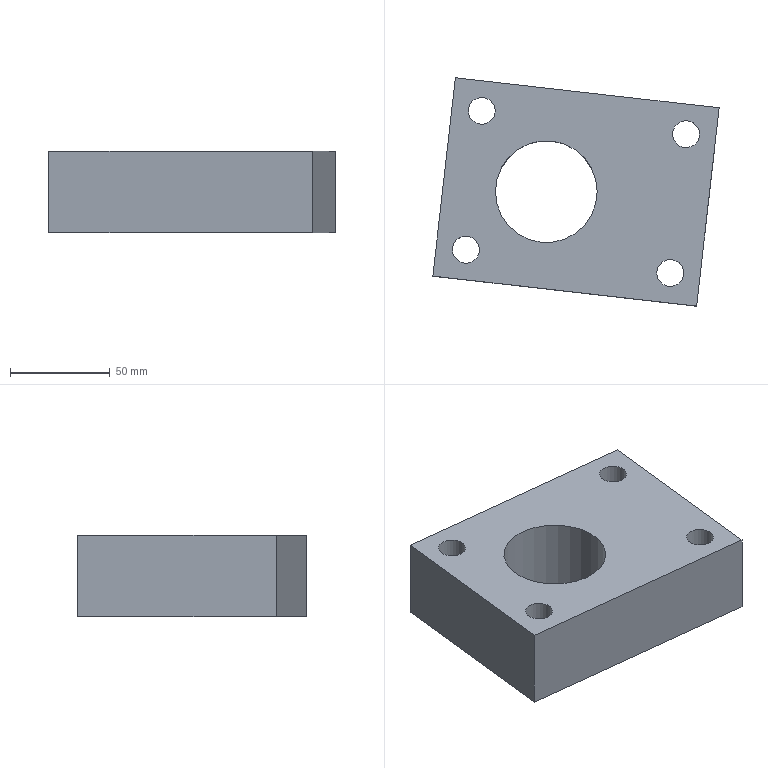Part | NX | features solid 2 | 1 solid | 19 faces | box 143.465 x 114.413 x 41 mm | volume 427808 mm3 | plane 10 | cylinder 9 | commonest cylinder face diameters 13.5 x4 20 x4 51 x1
STEP:
#1=CARTESIAN_POINT('',(2599.823,-120.761,101.));
#2=VERTEX_POINT('',#1);
#3=CARTESIAN_POINT('',(2593.073,-120.761,101.));
#4=DIRECTION('',(0.,0.,-1.));
#5=DIRECTION('',(1.,0.,0.));
#6=AXIS2_PLACEMENT_3D('',#3,#4,#5);
#7=CIRCLE('',#6,6.75);
#8=EDGE_CURVE('',#2,#2,#7,.T.);
#9=ORIENTED_EDGE('',*,*,#8,.T.);
#10=EDGE_LOOP('',(#9));
#11=FACE_BOUND('',#10,.T.);
#12=CARTESIAN_POINT('',(2607.575,-52.73,101.));
#13=VERTEX_POINT('',#12);
#14=CARTESIAN_POINT('',(2600.998,-51.211,101.));
#15=DIRECTION('',(0.,0.,1.));
#16=DIRECTION('',(0.9744,-0.225,0.));
#17=AXIS2_PLACEMENT_3D('',#14,#15,#16);
#18=CIRCLE('',#17,6.75);
#19=EDGE_CURVE('',#13,#13,#18,.T.);
#20=ORIENTED_EDGE('',*,*,#19,.F.);
#21=EDGE_LOOP('',(#20));
#22=FACE_BOUND('',#21,.T.);
#23=CARTESIAN_POINT('',(2606.279,-137.363,101.));
#24=VERTEX_POINT('',#23);
#25=CARTESIAN_POINT('',(2474.134,-122.307,101.));
#26=VERTEX_POINT('',#25);
#27=CARTESIAN_POINT('',(2529.774,-128.646,101.));
#28=DIRECTION('',(-0.9936,0.1132,0.));
#29=VECTOR('',#28,1000.);
#30=LINE('',#27,#29);
#31=EDGE_CURVE('',#24,#26,#30,.T.);
#32=ORIENTED_EDGE('',*,*,#31,.F.);
#33=CARTESIAN_POINT('',(2617.599,-38.006,101.));
#34=VERTEX_POINT('',#33);
#35=CARTESIAN_POINT('',(2612.505,-82.717,101.));
#36=DIRECTION('',(-0.1132,-0.9936,0.));
#37=VECTOR('',#36,1000.);
#38=LINE('',#35,#37);
#39=EDGE_CURVE('',#34,#24,#38,.T.);
#40=ORIENTED_EDGE('',*,*,#39,.F.);
#41=CARTESIAN_POINT('',(2485.454,-22.95,101.));
#42=VERTEX_POINT('',#41);
#43=CARTESIAN_POINT('',(2541.094,-29.289,101.));
#44=DIRECTION('',(0.9936,-0.1132,0.));
#45=VECTOR('',#44,1000.);
#46=LINE('',#43,#45);
#47=EDGE_CURVE('',#42,#34,#46,.T.);
#48=ORIENTED_EDGE('',*,*,#47,.F.);
#49=CARTESIAN_POINT('',(2480.36,-67.661,101.));
#50=DIRECTION('',(0.1132,0.9936,0.));
#51=VECTOR('',#50,1000.);
#52=LINE('',#49,#51);
#53=EDGE_CURVE('',#26,#42,#52,.T.);
#54=ORIENTED_EDGE('',*,*,#53,.F.);
#55=EDGE_LOOP('',(#32,#40,#48,#54));
#56=FACE_BOUND('',#55,.T.);
#57=CARTESIAN_POINT('',(2556.5,-80.,101.));
#58=VERTEX_POINT('',#57);
#59=CARTESIAN_POINT('',(2531.,-80.,101.));
#60=DIRECTION('',(0.,0.,1.));
#61=DIRECTION('',(1.,0.,0.));
#62=AXIS2_PLACEMENT_3D('',#59,#60,#61);
#63=CIRCLE('',#62,25.5);
#64=EDGE_CURVE('',#58,#58,#63,.T.);
#65=ORIENTED_EDGE('',*,*,#64,.F.);
#66=EDGE_LOOP('',(#65));
#67=FACE_BOUND('',#66,.T.);
#68=CARTESIAN_POINT('',(2484.158,-107.583,101.));
#69=VERTEX_POINT('',#68);
#70=CARTESIAN_POINT('',(2490.735,-109.102,101.));
#71=DIRECTION('',(0.,0.,1.));
#72=DIRECTION('',(-0.9744,0.225,0.));
#73=AXIS2_PLACEMENT_3D('',#70,#71,#72);
#74=CIRCLE('',#73,6.75);
#75=EDGE_CURVE('',#69,#69,#74,.T.);
#76=ORIENTED_EDGE('',*,*,#75,.F.);
#77=EDGE_LOOP('',(#76));
#78=FACE_BOUND('',#77,.T.);
#79=CARTESIAN_POINT('',(2491.91,-39.552,101.));
#80=VERTEX_POINT('',#79);
#81=CARTESIAN_POINT('',(2498.66,-39.552,101.));
#82=DIRECTION('',(0.,0.,-1.));
#83=DIRECTION('',(-1.,0.,0.));
#84=AXIS2_PLACEMENT_3D('',#81,#82,#83);
#85=CIRCLE('',#84,6.75);
#86=EDGE_CURVE('',#80,#80,#85,.T.);
#87=ORIENTED_EDGE('',*,*,#86,.T.);
#88=EDGE_LOOP('',(#87));
#89=FACE_BOUND('',#88,.T.);
#90=CARTESIAN_POINT('',(282.5,193.,101.));
#91=DIRECTION('',(0.,0.,1.));
#92=DIRECTION('',(-1.,0.,0.));
#93=AXIS2_PLACEMENT_3D('',#90,#91,#92);
#94=PLANE('',#93);
#95=ADVANCED_FACE('',(#11,#22,#56,#67,#78,#89),#94,.T.);
#96=CARTESIAN_POINT('',(2603.073,-120.761,60.));
#97=VERTEX_POINT('',#96);
#98=CARTESIAN_POINT('',(2593.073,-120.761,60.));
#99=DIRECTION('',(0.,0.,1.));
#100=DIRECTION('',(1.,0.,0.));
#101=AXIS2_PLACEMENT_3D('',#98,#99,#100);
#102=CIRCLE('',#101,10.);
#103=EDGE_CURVE('',#97,#97,#102,.T.);
#104=ORIENTED_EDGE('',*,*,#103,.T.);
#105=EDGE_LOOP('',(#104));
#106=FACE_BOUND('',#105,.T.);
#107=CARTESIAN_POINT('',(2610.741,-53.461,60.));
#108=VERTEX_POINT('',#107);
#109=CARTESIAN_POINT('',(2600.998,-51.211,60.));
#110=DIRECTION('',(0.,0.,-1.));
#111=DIRECTION('',(0.9744,-0.225,0.));
#112=AXIS2_PLACEMENT_3D('',#109,#110,#111);
#113=CIRCLE('',#112,10.);
#114=EDGE_CURVE('',#108,#108,#113,.T.);
#115=ORIENTED_EDGE('',*,*,#114,.F.);
#116=EDGE_LOOP('',(#115));
#117=FACE_BOUND('',#116,.T.);
#118=CARTESIAN_POINT('',(2606.279,-137.363,60.));
#119=VERTEX_POINT('',#118);
#120=CARTESIAN_POINT('',(2617.599,-38.006,60.));
#121=VERTEX_POINT('',#120);
#122=CARTESIAN_POINT('',(2612.505,-82.717,60.));
#123=DIRECTION('',(0.1132,0.9936,0.));
#124=VECTOR('',#123,1000.);
#125=LINE('',#122,#124);
#126=EDGE_CURVE('',#119,#121,#125,.T.);
#127=ORIENTED_EDGE('',*,*,#126,.F.);
#128=CARTESIAN_POINT('',(2474.134,-122.307,60.));
#129=VERTEX_POINT('',#128);
#130=CARTESIAN_POINT('',(2529.774,-128.646,60.));
#131=DIRECTION('',(0.9936,-0.1132,0.));
#132=VECTOR('',#131,1000.);
#133=LINE('',#130,#132);
#134=EDGE_CURVE('',#129,#119,#133,.T.);
#135=ORIENTED_EDGE('',*,*,#134,.F.);
#136=CARTESIAN_POINT('',(2485.454,-22.95,60.));
#137=VERTEX_POINT('',#136);
#138=CARTESIAN_POINT('',(2480.36,-67.661,60.));
#139=DIRECTION('',(-0.1132,-0.9936,0.));
#140=VECTOR('',#139,1000.);
#141=LINE('',#138,#140);
#142=EDGE_CURVE('',#137,#129,#141,.T.);
#143=ORIENTED_EDGE('',*,*,#142,.F.);
#144=CARTESIAN_POINT('',(2541.094,-29.289,60.));
#145=DIRECTION('',(-0.9936,0.1132,0.));
#146=VECTOR('',#145,1000.);
#147=LINE('',#144,#146);
#148=EDGE_CURVE('',#121,#137,#147,.T.);
#149=ORIENTED_EDGE('',*,*,#148,.F.);
#150=EDGE_LOOP('',(#127,#135,#143,#149));
#151=FACE_BOUND('',#150,.T.);
#152=CARTESIAN_POINT('',(2556.5,-80.,60.));
#153=VERTEX_POINT('',#152);
#154=CARTESIAN_POINT('',(2531.,-80.,60.));
#155=DIRECTION('',(0.,0.,-1.));
#156=DIRECTION('',(1.,0.,0.));
#157=AXIS2_PLACEMENT_3D('',#154,#155,#156);
#158=CIRCLE('',#157,25.5);
#159=EDGE_CURVE('',#153,#153,#158,.T.);
#160=ORIENTED_EDGE('',*,*,#159,.F.);
#161=EDGE_LOOP('',(#160));
#162=FACE_BOUND('',#161,.T.);
#163=CARTESIAN_POINT('',(2480.992,-106.852,60.));
#164=VERTEX_POINT('',#163);
#165=CARTESIAN_POINT('',(2490.735,-109.102,60.));
#166=DIRECTION('',(0.,0.,-1.));
#167=DIRECTION('',(-0.9744,0.225,0.));
#168=AXIS2_PLACEMENT_3D('',#165,#166,#167);
#169=CIRCLE('',#168,10.);
#170=EDGE_CURVE('',#164,#164,#169,.T.);
#171=ORIENTED_EDGE('',*,*,#170,.F.);
#172=EDGE_LOOP('',(#171));
#173=FACE_BOUND('',#172,.T.);
#174=CARTESIAN_POINT('',(2488.66,-39.552,60.));
#175=VERTEX_POINT('',#174);
#176=CARTESIAN_POINT('',(2498.66,-39.552,60.));
#177=DIRECTION('',(0.,0.,1.));
#178=DIRECTION('',(-1.,0.,0.));
#179=AXIS2_PLACEMENT_3D('',#176,#177,#178);
#180=CIRCLE('',#179,10.);
#181=EDGE_CURVE('',#175,#175,#180,.T.);
#182=ORIENTED_EDGE('',*,*,#181,.T.);
#183=EDGE_LOOP('',(#182));
#184=FACE_BOUND('',#183,.T.);
#185=CARTESIAN_POINT('',(2658.641,-285.511,60.));
#186=DIRECTION('',(0.,0.,1.));
#187=DIRECTION('',(-1.,0.,0.));
#188=AXIS2_PLACEMENT_3D('',#185,#186,#187);
#189=PLANE('',#188);
#190=ADVANCED_FACE('',(#106,#117,#151,#162,#173,#184),#189,.F.);
#191=CARTESIAN_POINT('',(2606.279,-137.363,-10.));
#192=DIRECTION('',(0.,0.,1.));
#193=VECTOR('',#192,1000.);
#194=LINE('',#191,#193);
#195=EDGE_CURVE('',#119,#24,#194,.T.);
#196=ORIENTED_EDGE('',*,*,#195,.T.);
#197=ORIENTED_EDGE('',*,*,#31,.T.);
#198=CARTESIAN_POINT('',(2474.134,-122.307,-10.));
#199=DIRECTION('',(0.,0.,1.));
#200=VECTOR('',#199,1000.);
#201=LINE('',#198,#200);
#202=EDGE_CURVE('',#129,#26,#201,.T.);
#203=ORIENTED_EDGE('',*,*,#202,.F.);
#204=ORIENTED_EDGE('',*,*,#134,.T.);
#205=EDGE_LOOP('',(#196,#197,#203,#204));
#206=FACE_BOUND('',#205,.T.);
#207=CARTESIAN_POINT('',(2529.774,-128.646,-10.));
#208=DIRECTION('',(-0.1132,-0.9936,0.));
#209=DIRECTION('',(-0.9936,0.1132,0.));
#210=AXIS2_PLACEMENT_3D('',#207,#208,#209);
#211=PLANE('',#210);
#212=ADVANCED_FACE('',(#206),#211,.T.);
#213=ORIENTED_EDGE('',*,*,#202,.T.);
#214=ORIENTED_EDGE('',*,*,#53,.T.);
#215=CARTESIAN_POINT('',(2485.454,-22.95,-10.));
#216=DIRECTION('',(0.,0.,1.));
#217=VECTOR('',#216,1000.);
#218=LINE('',#215,#217);
#219=EDGE_CURVE('',#137,#42,#218,.T.);
#220=ORIENTED_EDGE('',*,*,#219,.F.);
#221=ORIENTED_EDGE('',*,*,#142,.T.);
#222=EDGE_LOOP('',(#213,#214,#220,#221));
#223=FACE_BOUND('',#222,.T.);
#224=CARTESIAN_POINT('',(2480.36,-67.661,-10.));
#225=DIRECTION('',(-0.9936,0.1132,0.));
#226=DIRECTION('',(0.1132,0.9936,0.));
#227=AXIS2_PLACEMENT_3D('',#224,#225,#226);
#228=PLANE('',#227);
#229=ADVANCED_FACE('',(#223),#228,.T.);
#230=ORIENTED_EDGE('',*,*,#219,.T.);
#231=ORIENTED_EDGE('',*,*,#47,.T.);
#232=CARTESIAN_POINT('',(2617.599,-38.006,-10.));
#233=DIRECTION('',(0.,0.,1.));
#234=VECTOR('',#233,1000.);
#235=LINE('',#232,#234);
#236=EDGE_CURVE('',#121,#34,#235,.T.);
#237=ORIENTED_EDGE('',*,*,#236,.F.);
#238=ORIENTED_EDGE('',*,*,#148,.T.);
#239=EDGE_LOOP('',(#230,#231,#237,#238));
#240=FACE_BOUND('',#239,.T.);
#241=CARTESIAN_POINT('',(2541.094,-29.289,-10.));
#242=DIRECTION('',(0.1132,0.9936,0.));
#243=DIRECTION('',(0.9936,-0.1132,0.));
#244=AXIS2_PLACEMENT_3D('',#241,#242,#243);
#245=PLANE('',#244);
#246=ADVANCED_FACE('',(#240),#245,.T.);
#247=ORIENTED_EDGE('',*,*,#126,.T.);
#248=ORIENTED_EDGE('',*,*,#236,.T.);
#249=ORIENTED_EDGE('',*,*,#39,.T.);
#250=ORIENTED_EDGE('',*,*,#195,.F.);
#251=EDGE_LOOP('',(#247,#248,#249,#250));
#252=FACE_BOUND('',#251,.T.);
#253=CARTESIAN_POINT('',(2612.505,-82.717,-10.));
#254=DIRECTION('',(0.9936,-0.1132,0.));
#255=DIRECTION('',(-0.1132,-0.9936,0.));
#256=AXIS2_PLACEMENT_3D('',#253,#254,#255);
#257=PLANE('',#256);
#258=ADVANCED_FACE('',(#252),#257,.T.);
#259=ORIENTED_EDGE('',*,*,#64,.T.);
#260=EDGE_LOOP('',(#259));
#261=FACE_BOUND('',#260,.T.);
#262=ORIENTED_EDGE('',*,*,#159,.T.);
#263=EDGE_LOOP('',(#262));
#264=FACE_BOUND('',#263,.T.);
#265=CARTESIAN_POINT('',(2531.,-80.,-101.));
#266=DIRECTION('',(0.,0.,1.));
#267=DIRECTION('',(-1.,0.,0.));
#268=AXIS2_PLACEMENT_3D('',#265,#266,#267);
#269=CYLINDRICAL_SURFACE('',#268,25.5);
#270=ADVANCED_FACE('',(#261,#264),#269,.F.);
#271=CARTESIAN_POINT('',(2607.575,-52.73,75.));
#272=VERTEX_POINT('',#271);
#273=CARTESIAN_POINT('',(2600.998,-51.211,75.));
#274=DIRECTION('',(0.,0.,-1.));
#275=DIRECTION('',(0.9744,-0.225,0.));
#276=AXIS2_PLACEMENT_3D('',#273,#274,#275);
#277=CIRCLE('',#276,6.75);
#278=EDGE_CURVE('',#272,#272,#277,.T.);
#279=ORIENTED_EDGE('',*,*,#278,.T.);
#280=EDGE_LOOP('',(#279));
#281=FACE_BOUND('',#280,.T.);
#282=ORIENTED_EDGE('',*,*,#19,.T.);
#283=EDGE_LOOP('',(#282));
#284=FACE_BOUND('',#283,.T.);
#285=CARTESIAN_POINT('',(2600.998,-51.211,60.));
#286=DIRECTION('',(0.,0.,1.));
#287=DIRECTION('',(-0.9744,0.225,0.));
#288=AXIS2_PLACEMENT_3D('',#285,#286,#287);
#289=CYLINDRICAL_SURFACE('',#288,6.75);
#290=ADVANCED_FACE('',(#281,#284),#289,.F.);
#291=ORIENTED_EDGE('',*,*,#278,.F.);
#292=EDGE_LOOP('',(#291));
#293=FACE_BOUND('',#292,.T.);
#294=CARTESIAN_POINT('',(2610.741,-53.461,75.));
#295=VERTEX_POINT('',#294);
#296=CARTESIAN_POINT('',(2600.998,-51.211,75.));
#297=DIRECTION('',(0.,0.,-1.));
#298=DIRECTION('',(0.9744,-0.225,0.));
#299=AXIS2_PLACEMENT_3D('',#296,#297,#298);
#300=CIRCLE('',#299,10.);
#301=EDGE_CURVE('',#295,#295,#300,.T.);
#302=ORIENTED_EDGE('',*,*,#301,.T.);
#303=EDGE_LOOP('',(#302));
#304=FACE_BOUND('',#303,.T.);
#305=CARTESIAN_POINT('',(2600.998,-51.211,75.));
#306=DIRECTION('',(0.,0.,1.));
#307=DIRECTION('',(-0.9744,0.225,0.));
#308=AXIS2_PLACEMENT_3D('',#305,#306,#307);
#309=PLANE('',#308);
#310=ADVANCED_FACE('',(#293,#304),#309,.F.);
#311=ORIENTED_EDGE('',*,*,#301,.F.);
#312=EDGE_LOOP('',(#311));
#313=FACE_BOUND('',#312,.T.);
#314=ORIENTED_EDGE('',*,*,#114,.T.);
#315=EDGE_LOOP('',(#314));
#316=FACE_BOUND('',#315,.T.);
#317=CARTESIAN_POINT('',(2600.998,-51.211,60.));
#318=DIRECTION('',(0.,0.,1.));
#319=DIRECTION('',(-0.9744,0.225,0.));
#320=AXIS2_PLACEMENT_3D('',#317,#318,#319);
#321=CYLINDRICAL_SURFACE('',#320,10.);
#322=ADVANCED_FACE('',(#313,#316),#321,.F.);
#323=CARTESIAN_POINT('',(2599.823,-120.761,75.));
#324=VERTEX_POINT('',#323);
#325=CARTESIAN_POINT('',(2593.073,-120.761,75.));
#326=DIRECTION('',(0.,0.,1.));
#327=DIRECTION('',(1.,0.,0.));
#328=AXIS2_PLACEMENT_3D('',#325,#326,#327);
#329=CIRCLE('',#328,6.75);
#330=EDGE_CURVE('',#324,#324,#329,.T.);
#331=ORIENTED_EDGE('',*,*,#330,.F.);
#332=EDGE_LOOP('',(#331));
#333=FACE_BOUND('',#332,.T.);
#334=ORIENTED_EDGE('',*,*,#8,.F.);
#335=EDGE_LOOP('',(#334));
#336=FACE_BOUND('',#335,.T.);
#337=CARTESIAN_POINT('',(2593.073,-120.761,60.));
#338=DIRECTION('',(0.,0.,1.));
#339=DIRECTION('',(-1.,0.,0.));
#340=AXIS2_PLACEMENT_3D('',#337,#338,#339);
#341=CYLINDRICAL_SURFACE('',#340,6.75);
#342=ADVANCED_FACE('',(#333,#336),#341,.F.);
#343=ORIENTED_EDGE('',*,*,#330,.T.);
#344=EDGE_LOOP('',(#343));
#345=FACE_BOUND('',#344,.T.);
#346=CARTESIAN_POINT('',(2603.073,-120.761,75.));
#347=VERTEX_POINT('',#346);
#348=CARTESIAN_POINT('',(2593.073,-120.761,75.));
#349=DIRECTION('',(0.,0.,1.));
#350=DIRECTION('',(1.,0.,0.));
#351=AXIS2_PLACEMENT_3D('',#348,#349,#350);
#352=CIRCLE('',#351,10.);
#353=EDGE_CURVE('',#347,#347,#352,.T.);
#354=ORIENTED_EDGE('',*,*,#353,.F.);
#355=EDGE_LOOP('',(#354));
#356=FACE_BOUND('',#355,.T.);
#357=CARTESIAN_POINT('',(2593.073,-120.761,75.));
#358=DIRECTION('',(0.,0.,1.));
#359=DIRECTION('',(-1.,0.,0.));
#360=AXIS2_PLACEMENT_3D('',#357,#358,#359);
#361=PLANE('',#360);
#362=ADVANCED_FACE('',(#345,#356),#361,.F.);
#363=ORIENTED_EDGE('',*,*,#353,.T.);
#364=EDGE_LOOP('',(#363));
#365=FACE_BOUND('',#364,.T.);
#366=ORIENTED_EDGE('',*,*,#103,.F.);
#367=EDGE_LOOP('',(#366));
#368=FACE_BOUND('',#367,.T.);
#369=CARTESIAN_POINT('',(2593.073,-120.761,60.));
#370=DIRECTION('',(0.,0.,1.));
#371=DIRECTION('',(-1.,0.,0.));
#372=AXIS2_PLACEMENT_3D('',#369,#370,#371);
#373=CYLINDRICAL_SURFACE('',#372,10.);
#374=ADVANCED_FACE('',(#365,#368),#373,.F.);
#375=CARTESIAN_POINT('',(2484.158,-107.583,75.));
#376=VERTEX_POINT('',#375);
#377=CARTESIAN_POINT('',(2490.735,-109.102,75.));
#378=DIRECTION('',(0.,0.,-1.));
#379=DIRECTION('',(-0.9744,0.225,0.));
#380=AXIS2_PLACEMENT_3D('',#377,#378,#379);
#381=CIRCLE('',#380,6.75);
#382=EDGE_CURVE('',#376,#376,#381,.T.);
#383=ORIENTED_EDGE('',*,*,#382,.T.);
#384=EDGE_LOOP('',(#383));
#385=FACE_BOUND('',#384,.T.);
#386=ORIENTED_EDGE('',*,*,#75,.T.);
#387=EDGE_LOOP('',(#386));
#388=FACE_BOUND('',#387,.T.);
#389=CARTESIAN_POINT('',(2490.735,-109.102,60.));
#390=DIRECTION('',(0.,0.,1.));
#391=DIRECTION('',(0.9744,-0.225,0.));
#392=AXIS2_PLACEMENT_3D('',#389,#390,#391);
#393=CYLINDRICAL_SURFACE('',#392,6.75);
#394=ADVANCED_FACE('',(#385,#388),#393,.F.);
#395=ORIENTED_EDGE('',*,*,#382,.F.);
#396=EDGE_LOOP('',(#395));
#397=FACE_BOUND('',#396,.T.);
#398=CARTESIAN_POINT('',(2480.992,-106.852,75.));
#399=VERTEX_POINT('',#398);
#400=CARTESIAN_POINT('',(2490.735,-109.102,75.));
#401=DIRECTION('',(0.,0.,-1.));
#402=DIRECTION('',(-0.9744,0.225,0.));
#403=AXIS2_PLACEMENT_3D('',#400,#401,#402);
#404=CIRCLE('',#403,10.);
#405=EDGE_CURVE('',#399,#399,#404,.T.);
#406=ORIENTED_EDGE('',*,*,#405,.T.);
#407=EDGE_LOOP('',(#406));
#408=FACE_BOUND('',#407,.T.);
#409=CARTESIAN_POINT('',(2490.735,-109.102,75.));
#410=DIRECTION('',(0.,0.,1.));
#411=DIRECTION('',(0.9744,-0.225,0.));
#412=AXIS2_PLACEMENT_3D('',#409,#410,#411);
#413=PLANE('',#412);
#414=ADVANCED_FACE('',(#397,#408),#413,.F.);
#415=ORIENTED_EDGE('',*,*,#405,.F.);
#416=EDGE_LOOP('',(#415));
#417=FACE_BOUND('',#416,.T.);
#418=ORIENTED_EDGE('',*,*,#170,.T.);
#419=EDGE_LOOP('',(#418));
#420=FACE_BOUND('',#419,.T.);
#421=CARTESIAN_POINT('',(2490.735,-109.102,60.));
#422=DIRECTION('',(0.,0.,1.));
#423=DIRECTION('',(0.9744,-0.225,0.));
#424=AXIS2_PLACEMENT_3D('',#421,#422,#423);
#425=CYLINDRICAL_SURFACE('',#424,10.);
#426=ADVANCED_FACE('',(#417,#420),#425,.F.);
#427=CARTESIAN_POINT('',(2491.91,-39.552,75.));
#428=VERTEX_POINT('',#427);
#429=CARTESIAN_POINT('',(2498.66,-39.552,75.));
#430=DIRECTION('',(0.,0.,1.));
#431=DIRECTION('',(-1.,0.,0.));
#432=AXIS2_PLACEMENT_3D('',#429,#430,#431);
#433=CIRCLE('',#432,6.75);
#434=EDGE_CURVE('',#428,#428,#433,.T.);
#435=ORIENTED_EDGE('',*,*,#434,.F.);
#436=EDGE_LOOP('',(#435));
#437=FACE_BOUND('',#436,.T.);
#438=ORIENTED_EDGE('',*,*,#86,.F.);
#439=EDGE_LOOP('',(#438));
#440=FACE_BOUND('',#439,.T.);
#441=CARTESIAN_POINT('',(2498.66,-39.552,60.));
#442=DIRECTION('',(0.,0.,1.));
#443=DIRECTION('',(1.,0.,0.));
#444=AXIS2_PLACEMENT_3D('',#441,#442,#443);
#445=CYLINDRICAL_SURFACE('',#444,6.75);
#446=ADVANCED_FACE('',(#437,#440),#445,.F.);
#447=ORIENTED_EDGE('',*,*,#434,.T.);
#448=EDGE_LOOP('',(#447));
#449=FACE_BOUND('',#448,.T.);
#450=CARTESIAN_POINT('',(2488.66,-39.552,75.));
#451=VERTEX_POINT('',#450);
#452=CARTESIAN_POINT('',(2498.66,-39.552,75.));
#453=DIRECTION('',(0.,0.,1.));
#454=DIRECTION('',(-1.,0.,0.));
#455=AXIS2_PLACEMENT_3D('',#452,#453,#454);
#456=CIRCLE('',#455,10.);
#457=EDGE_CURVE('',#451,#451,#456,.T.);
#458=ORIENTED_EDGE('',*,*,#457,.F.);
#459=EDGE_LOOP('',(#458));
#460=FACE_BOUND('',#459,.T.);
#461=CARTESIAN_POINT('',(2498.66,-39.552,75.));
#462=DIRECTION('',(0.,0.,1.));
#463=DIRECTION('',(1.,0.,0.));
#464=AXIS2_PLACEMENT_3D('',#461,#462,#463);
#465=PLANE('',#464);
#466=ADVANCED_FACE('',(#449,#460),#465,.F.);
#467=ORIENTED_EDGE('',*,*,#457,.T.);
#468=EDGE_LOOP('',(#467));
#469=FACE_BOUND('',#468,.T.);
#470=ORIENTED_EDGE('',*,*,#181,.F.);
#471=EDGE_LOOP('',(#470));
#472=FACE_BOUND('',#471,.T.);
#473=CARTESIAN_POINT('',(2498.66,-39.552,60.));
#474=DIRECTION('',(0.,0.,1.));
#475=DIRECTION('',(1.,0.,0.));
#476=AXIS2_PLACEMENT_3D('',#473,#474,#475);
#477=CYLINDRICAL_SURFACE('',#476,10.);
#478=ADVANCED_FACE('',(#469,#472),#477,.F.);
#479=CLOSED_SHELL('',(#95,#190,#212,#229,#246,#258,#270,#290,#310,#322,#342,#362,#374,#394,#414,#426,#446,#466,#478));
#480=MANIFOLD_SOLID_BREP('',#479);
#481=(LENGTH_UNIT()NAMED_UNIT(*)SI_UNIT(.MILLI.,.METRE.));
#482=UNCERTAINTY_MEASURE_WITH_UNIT(LENGTH_MEASURE(0.00001),#481,'','');
#483=(NAMED_UNIT(*)PLANE_ANGLE_UNIT()SI_UNIT($,.RADIAN.));
#484=(NAMED_UNIT(*)SI_UNIT($,.STERADIAN.)SOLID_ANGLE_UNIT());
#485=(GEOMETRIC_REPRESENTATION_CONTEXT(3)GLOBAL_UNCERTAINTY_ASSIGNED_CONTEXT((#482))GLOBAL_UNIT_ASSIGNED_CONTEXT((#481,#483,#484))REPRESENTATION_CONTEXT('',''));
#486=ADVANCED_BREP_SHAPE_REPRESENTATION('',(#480),#485);